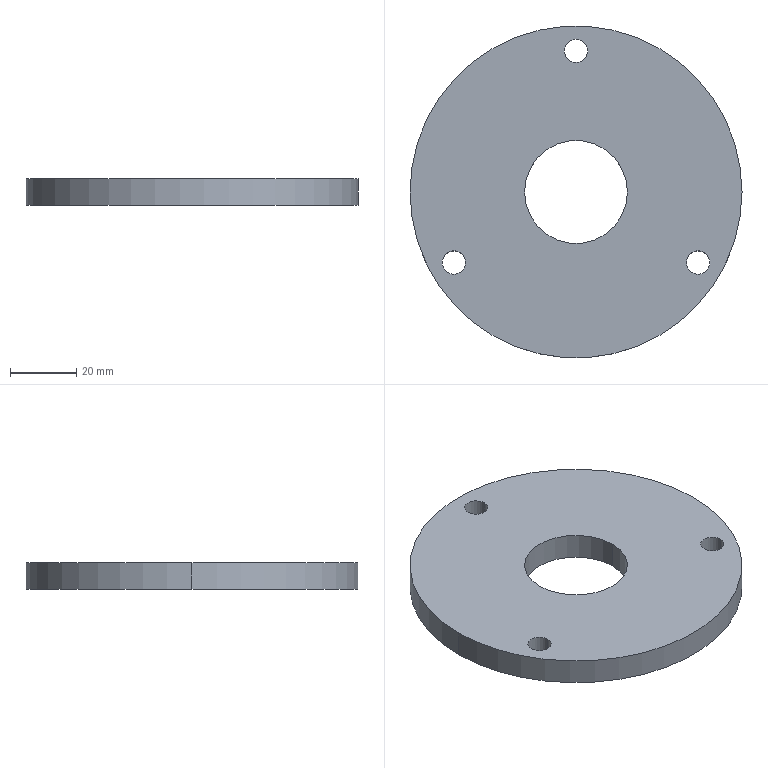Part | SolidWorks | features Extrusion 1 | 1 solid | 12 faces | box 100 x 100 x 8 mm | volume 55870 mm3 | cylinder 10 | plane 2 | commonest cylinder face diameters 7 x6 31 x2 100 x2
STEP:
#1=CARTESIAN_POINT('',(-15.5,0.,8.));
#2=VERTEX_POINT('',#1);
#3=CARTESIAN_POINT('',(15.5,0.,8.));
#4=VERTEX_POINT('',#3);
#5=CARTESIAN_POINT('',(0.,0.,8.));
#6=DIRECTION('',(0.,0.,1.));
#7=DIRECTION('',(1.,0.,0.));
#8=AXIS2_PLACEMENT_3D('',#5,#6,#7);
#9=CIRCLE('',#8,15.5);
#10=EDGE_CURVE('',#2,#4,#9,.T.);
#11=ORIENTED_EDGE('',*,*,#10,.T.);
#12=CARTESIAN_POINT('',(15.5,0.,0.));
#13=VERTEX_POINT('',#12);
#14=CARTESIAN_POINT('',(15.5,0.,8.));
#15=DIRECTION('',(0.,0.,-1.));
#16=VECTOR('',#15,1000.);
#17=LINE('',#14,#16);
#18=EDGE_CURVE('',#4,#13,#17,.T.);
#19=ORIENTED_EDGE('',*,*,#18,.T.);
#20=CARTESIAN_POINT('',(-15.5,0.,0.));
#21=VERTEX_POINT('',#20);
#22=CARTESIAN_POINT('',(0.,0.,0.));
#23=DIRECTION('',(0.,0.,1.));
#24=DIRECTION('',(1.,0.,0.));
#25=AXIS2_PLACEMENT_3D('',#22,#23,#24);
#26=CIRCLE('',#25,15.5);
#27=EDGE_CURVE('',#21,#13,#26,.T.);
#28=ORIENTED_EDGE('',*,*,#27,.F.);
#29=CARTESIAN_POINT('',(-15.5,0.,8.));
#30=DIRECTION('',(0.,0.,-1.));
#31=VECTOR('',#30,1000.);
#32=LINE('',#29,#31);
#33=EDGE_CURVE('',#2,#21,#32,.T.);
#34=ORIENTED_EDGE('',*,*,#33,.F.);
#35=EDGE_LOOP('',(#11,#19,#28,#34));
#36=FACE_OUTER_BOUND('',#35,.T.);
#37=CARTESIAN_POINT('',(0.,0.,8.));
#38=DIRECTION('',(0.,0.,-1.));
#39=DIRECTION('',(-1.,0.,0.));
#40=AXIS2_PLACEMENT_3D('',#37,#38,#39);
#41=CYLINDRICAL_SURFACE('',#40,15.5);
#42=ADVANCED_FACE('',(#36),#41,.F.);
#43=CARTESIAN_POINT('',(33.306,-21.25,8.));
#44=VERTEX_POINT('',#43);
#45=CARTESIAN_POINT('',(40.306,-21.25,8.));
#46=VERTEX_POINT('',#45);
#47=CARTESIAN_POINT('',(36.806,-21.25,8.));
#48=DIRECTION('',(0.,0.,1.));
#49=DIRECTION('',(1.,0.,0.));
#50=AXIS2_PLACEMENT_3D('',#47,#48,#49);
#51=CIRCLE('',#50,3.5);
#52=EDGE_CURVE('',#44,#46,#51,.T.);
#53=ORIENTED_EDGE('',*,*,#52,.T.);
#54=CARTESIAN_POINT('',(40.306,-21.25,0.));
#55=VERTEX_POINT('',#54);
#56=CARTESIAN_POINT('',(40.306,-21.25,8.));
#57=DIRECTION('',(0.,0.,-1.));
#58=VECTOR('',#57,1000.);
#59=LINE('',#56,#58);
#60=EDGE_CURVE('',#46,#55,#59,.T.);
#61=ORIENTED_EDGE('',*,*,#60,.T.);
#62=CARTESIAN_POINT('',(33.306,-21.25,0.));
#63=VERTEX_POINT('',#62);
#64=CARTESIAN_POINT('',(36.806,-21.25,0.));
#65=DIRECTION('',(0.,0.,1.));
#66=DIRECTION('',(1.,0.,0.));
#67=AXIS2_PLACEMENT_3D('',#64,#65,#66);
#68=CIRCLE('',#67,3.5);
#69=EDGE_CURVE('',#63,#55,#68,.T.);
#70=ORIENTED_EDGE('',*,*,#69,.F.);
#71=CARTESIAN_POINT('',(33.306,-21.25,8.));
#72=DIRECTION('',(0.,0.,-1.));
#73=VECTOR('',#72,1000.);
#74=LINE('',#71,#73);
#75=EDGE_CURVE('',#44,#63,#74,.T.);
#76=ORIENTED_EDGE('',*,*,#75,.F.);
#77=EDGE_LOOP('',(#53,#61,#70,#76));
#78=FACE_OUTER_BOUND('',#77,.T.);
#79=CARTESIAN_POINT('',(36.806,-21.25,8.));
#80=DIRECTION('',(0.,0.,-1.));
#81=DIRECTION('',(-1.,0.,0.));
#82=AXIS2_PLACEMENT_3D('',#79,#80,#81);
#83=CYLINDRICAL_SURFACE('',#82,3.5);
#84=ADVANCED_FACE('',(#78),#83,.F.);
#85=CARTESIAN_POINT('',(-40.306,-21.25,8.));
#86=VERTEX_POINT('',#85);
#87=CARTESIAN_POINT('',(-33.306,-21.25,8.));
#88=VERTEX_POINT('',#87);
#89=CARTESIAN_POINT('',(-36.806,-21.25,8.));
#90=DIRECTION('',(0.,0.,1.));
#91=DIRECTION('',(1.,0.,0.));
#92=AXIS2_PLACEMENT_3D('',#89,#90,#91);
#93=CIRCLE('',#92,3.5);
#94=EDGE_CURVE('',#86,#88,#93,.T.);
#95=ORIENTED_EDGE('',*,*,#94,.T.);
#96=CARTESIAN_POINT('',(-33.306,-21.25,0.));
#97=VERTEX_POINT('',#96);
#98=CARTESIAN_POINT('',(-33.306,-21.25,8.));
#99=DIRECTION('',(0.,0.,-1.));
#100=VECTOR('',#99,1000.);
#101=LINE('',#98,#100);
#102=EDGE_CURVE('',#88,#97,#101,.T.);
#103=ORIENTED_EDGE('',*,*,#102,.T.);
#104=CARTESIAN_POINT('',(-40.306,-21.25,0.));
#105=VERTEX_POINT('',#104);
#106=CARTESIAN_POINT('',(-36.806,-21.25,0.));
#107=DIRECTION('',(0.,0.,1.));
#108=DIRECTION('',(1.,0.,0.));
#109=AXIS2_PLACEMENT_3D('',#106,#107,#108);
#110=CIRCLE('',#109,3.5);
#111=EDGE_CURVE('',#105,#97,#110,.T.);
#112=ORIENTED_EDGE('',*,*,#111,.F.);
#113=CARTESIAN_POINT('',(-40.306,-21.25,8.));
#114=DIRECTION('',(0.,0.,-1.));
#115=VECTOR('',#114,1000.);
#116=LINE('',#113,#115);
#117=EDGE_CURVE('',#86,#105,#116,.T.);
#118=ORIENTED_EDGE('',*,*,#117,.F.);
#119=EDGE_LOOP('',(#95,#103,#112,#118));
#120=FACE_OUTER_BOUND('',#119,.T.);
#121=CARTESIAN_POINT('',(-36.806,-21.25,8.));
#122=DIRECTION('',(0.,0.,-1.));
#123=DIRECTION('',(-1.,0.,0.));
#124=AXIS2_PLACEMENT_3D('',#121,#122,#123);
#125=CYLINDRICAL_SURFACE('',#124,3.5);
#126=ADVANCED_FACE('',(#120),#125,.F.);
#127=CARTESIAN_POINT('',(-3.5,42.5,8.));
#128=VERTEX_POINT('',#127);
#129=CARTESIAN_POINT('',(3.5,42.5,8.));
#130=VERTEX_POINT('',#129);
#131=CARTESIAN_POINT('',(0.,42.5,8.));
#132=DIRECTION('',(0.,0.,1.));
#133=DIRECTION('',(1.,0.,0.));
#134=AXIS2_PLACEMENT_3D('',#131,#132,#133);
#135=CIRCLE('',#134,3.5);
#136=EDGE_CURVE('',#128,#130,#135,.T.);
#137=ORIENTED_EDGE('',*,*,#136,.T.);
#138=CARTESIAN_POINT('',(3.5,42.5,0.));
#139=VERTEX_POINT('',#138);
#140=CARTESIAN_POINT('',(3.5,42.5,8.));
#141=DIRECTION('',(0.,0.,-1.));
#142=VECTOR('',#141,1000.);
#143=LINE('',#140,#142);
#144=EDGE_CURVE('',#130,#139,#143,.T.);
#145=ORIENTED_EDGE('',*,*,#144,.T.);
#146=CARTESIAN_POINT('',(-3.5,42.5,0.));
#147=VERTEX_POINT('',#146);
#148=CARTESIAN_POINT('',(0.,42.5,0.));
#149=DIRECTION('',(0.,0.,1.));
#150=DIRECTION('',(1.,0.,0.));
#151=AXIS2_PLACEMENT_3D('',#148,#149,#150);
#152=CIRCLE('',#151,3.5);
#153=EDGE_CURVE('',#147,#139,#152,.T.);
#154=ORIENTED_EDGE('',*,*,#153,.F.);
#155=CARTESIAN_POINT('',(-3.5,42.5,8.));
#156=DIRECTION('',(0.,0.,-1.));
#157=VECTOR('',#156,1000.);
#158=LINE('',#155,#157);
#159=EDGE_CURVE('',#128,#147,#158,.T.);
#160=ORIENTED_EDGE('',*,*,#159,.F.);
#161=EDGE_LOOP('',(#137,#145,#154,#160));
#162=FACE_OUTER_BOUND('',#161,.T.);
#163=CARTESIAN_POINT('',(0.,42.5,8.));
#164=DIRECTION('',(0.,0.,-1.));
#165=DIRECTION('',(-1.,0.,0.));
#166=AXIS2_PLACEMENT_3D('',#163,#164,#165);
#167=CYLINDRICAL_SURFACE('',#166,3.5);
#168=ADVANCED_FACE('',(#162),#167,.F.);
#169=CARTESIAN_POINT('',(50.,0.,8.));
#170=VERTEX_POINT('',#169);
#171=CARTESIAN_POINT('',(-50.,0.,8.));
#172=VERTEX_POINT('',#171);
#173=CARTESIAN_POINT('',(0.,0.,8.));
#174=DIRECTION('',(0.,0.,1.));
#175=DIRECTION('',(1.,0.,0.));
#176=AXIS2_PLACEMENT_3D('',#173,#174,#175);
#177=CIRCLE('',#176,50.);
#178=EDGE_CURVE('',#170,#172,#177,.T.);
#179=ORIENTED_EDGE('',*,*,#178,.F.);
#180=CARTESIAN_POINT('',(50.,0.,0.));
#181=VERTEX_POINT('',#180);
#182=CARTESIAN_POINT('',(50.,0.,8.));
#183=DIRECTION('',(0.,0.,-1.));
#184=VECTOR('',#183,1000.);
#185=LINE('',#182,#184);
#186=EDGE_CURVE('',#170,#181,#185,.T.);
#187=ORIENTED_EDGE('',*,*,#186,.T.);
#188=CARTESIAN_POINT('',(-50.,0.,0.));
#189=VERTEX_POINT('',#188);
#190=CARTESIAN_POINT('',(0.,0.,0.));
#191=DIRECTION('',(0.,0.,1.));
#192=DIRECTION('',(1.,0.,0.));
#193=AXIS2_PLACEMENT_3D('',#190,#191,#192);
#194=CIRCLE('',#193,50.);
#195=EDGE_CURVE('',#181,#189,#194,.T.);
#196=ORIENTED_EDGE('',*,*,#195,.T.);
#197=CARTESIAN_POINT('',(-50.,0.,8.));
#198=DIRECTION('',(0.,0.,-1.));
#199=VECTOR('',#198,1000.);
#200=LINE('',#197,#199);
#201=EDGE_CURVE('',#172,#189,#200,.T.);
#202=ORIENTED_EDGE('',*,*,#201,.F.);
#203=EDGE_LOOP('',(#179,#187,#196,#202));
#204=FACE_OUTER_BOUND('',#203,.T.);
#205=CARTESIAN_POINT('',(0.,0.,8.));
#206=DIRECTION('',(0.,0.,-1.));
#207=DIRECTION('',(-1.,0.,0.));
#208=AXIS2_PLACEMENT_3D('',#205,#206,#207);
#209=CYLINDRICAL_SURFACE('',#208,50.);
#210=ADVANCED_FACE('',(#204),#209,.T.);
#211=ORIENTED_EDGE('',*,*,#52,.F.);
#212=CARTESIAN_POINT('',(36.806,-21.25,8.));
#213=DIRECTION('',(0.,0.,1.));
#214=DIRECTION('',(1.,0.,0.));
#215=AXIS2_PLACEMENT_3D('',#212,#213,#214);
#216=CIRCLE('',#215,3.5);
#217=EDGE_CURVE('',#46,#44,#216,.T.);
#218=ORIENTED_EDGE('',*,*,#217,.F.);
#219=EDGE_LOOP('',(#211,#218));
#220=FACE_BOUND('',#219,.T.);
#221=ORIENTED_EDGE('',*,*,#136,.F.);
#222=CARTESIAN_POINT('',(0.,42.5,8.));
#223=DIRECTION('',(0.,0.,1.));
#224=DIRECTION('',(1.,0.,0.));
#225=AXIS2_PLACEMENT_3D('',#222,#223,#224);
#226=CIRCLE('',#225,3.5);
#227=EDGE_CURVE('',#130,#128,#226,.T.);
#228=ORIENTED_EDGE('',*,*,#227,.F.);
#229=EDGE_LOOP('',(#221,#228));
#230=FACE_BOUND('',#229,.T.);
#231=CARTESIAN_POINT('',(0.,0.,8.));
#232=DIRECTION('',(0.,0.,1.));
#233=DIRECTION('',(1.,0.,0.));
#234=AXIS2_PLACEMENT_3D('',#231,#232,#233);
#235=CIRCLE('',#234,50.);
#236=EDGE_CURVE('',#172,#170,#235,.T.);
#237=ORIENTED_EDGE('',*,*,#236,.T.);
#238=ORIENTED_EDGE('',*,*,#178,.T.);
#239=EDGE_LOOP('',(#237,#238));
#240=FACE_OUTER_BOUND('',#239,.T.);
#241=ORIENTED_EDGE('',*,*,#94,.F.);
#242=CARTESIAN_POINT('',(-36.806,-21.25,8.));
#243=DIRECTION('',(0.,0.,1.));
#244=DIRECTION('',(1.,0.,0.));
#245=AXIS2_PLACEMENT_3D('',#242,#243,#244);
#246=CIRCLE('',#245,3.5);
#247=EDGE_CURVE('',#88,#86,#246,.T.);
#248=ORIENTED_EDGE('',*,*,#247,.F.);
#249=EDGE_LOOP('',(#241,#248));
#250=FACE_BOUND('',#249,.T.);
#251=ORIENTED_EDGE('',*,*,#10,.F.);
#252=CARTESIAN_POINT('',(0.,0.,8.));
#253=DIRECTION('',(0.,0.,1.));
#254=DIRECTION('',(1.,0.,0.));
#255=AXIS2_PLACEMENT_3D('',#252,#253,#254);
#256=CIRCLE('',#255,15.5);
#257=EDGE_CURVE('',#4,#2,#256,.T.);
#258=ORIENTED_EDGE('',*,*,#257,.F.);
#259=EDGE_LOOP('',(#251,#258));
#260=FACE_BOUND('',#259,.T.);
#261=CARTESIAN_POINT('',(0.,0.,8.));
#262=DIRECTION('',(0.,0.,1.));
#263=DIRECTION('',(1.,0.,0.));
#264=AXIS2_PLACEMENT_3D('',#261,#262,#263);
#265=PLANE('',#264);
#266=ADVANCED_FACE('',(#220,#230,#240,#250,#260),#265,.T.);
#267=CARTESIAN_POINT('',(0.,0.,0.));
#268=DIRECTION('',(0.,0.,1.));
#269=DIRECTION('',(1.,0.,0.));
#270=AXIS2_PLACEMENT_3D('',#267,#268,#269);
#271=CIRCLE('',#270,50.);
#272=EDGE_CURVE('',#189,#181,#271,.T.);
#273=ORIENTED_EDGE('',*,*,#272,.F.);
#274=ORIENTED_EDGE('',*,*,#195,.F.);
#275=EDGE_LOOP('',(#273,#274));
#276=FACE_OUTER_BOUND('',#275,.T.);
#277=ORIENTED_EDGE('',*,*,#153,.T.);
#278=CARTESIAN_POINT('',(0.,42.5,0.));
#279=DIRECTION('',(0.,0.,1.));
#280=DIRECTION('',(1.,0.,0.));
#281=AXIS2_PLACEMENT_3D('',#278,#279,#280);
#282=CIRCLE('',#281,3.5);
#283=EDGE_CURVE('',#139,#147,#282,.T.);
#284=ORIENTED_EDGE('',*,*,#283,.T.);
#285=EDGE_LOOP('',(#277,#284));
#286=FACE_BOUND('',#285,.T.);
#287=ORIENTED_EDGE('',*,*,#111,.T.);
#288=CARTESIAN_POINT('',(-36.806,-21.25,0.));
#289=DIRECTION('',(0.,0.,1.));
#290=DIRECTION('',(1.,0.,0.));
#291=AXIS2_PLACEMENT_3D('',#288,#289,#290);
#292=CIRCLE('',#291,3.5);
#293=EDGE_CURVE('',#97,#105,#292,.T.);
#294=ORIENTED_EDGE('',*,*,#293,.T.);
#295=EDGE_LOOP('',(#287,#294));
#296=FACE_BOUND('',#295,.T.);
#297=ORIENTED_EDGE('',*,*,#69,.T.);
#298=CARTESIAN_POINT('',(36.806,-21.25,0.));
#299=DIRECTION('',(0.,0.,1.));
#300=DIRECTION('',(1.,0.,0.));
#301=AXIS2_PLACEMENT_3D('',#298,#299,#300);
#302=CIRCLE('',#301,3.5);
#303=EDGE_CURVE('',#55,#63,#302,.T.);
#304=ORIENTED_EDGE('',*,*,#303,.T.);
#305=EDGE_LOOP('',(#297,#304));
#306=FACE_BOUND('',#305,.T.);
#307=ORIENTED_EDGE('',*,*,#27,.T.);
#308=CARTESIAN_POINT('',(0.,0.,0.));
#309=DIRECTION('',(0.,0.,1.));
#310=DIRECTION('',(1.,0.,0.));
#311=AXIS2_PLACEMENT_3D('',#308,#309,#310);
#312=CIRCLE('',#311,15.5);
#313=EDGE_CURVE('',#13,#21,#312,.T.);
#314=ORIENTED_EDGE('',*,*,#313,.T.);
#315=EDGE_LOOP('',(#307,#314));
#316=FACE_BOUND('',#315,.T.);
#317=CARTESIAN_POINT('',(0.,0.,0.));
#318=DIRECTION('',(0.,0.,1.));
#319=DIRECTION('',(1.,0.,0.));
#320=AXIS2_PLACEMENT_3D('',#317,#318,#319);
#321=PLANE('',#320);
#322=ADVANCED_FACE('',(#276,#286,#296,#306,#316),#321,.F.);
#323=ORIENTED_EDGE('',*,*,#186,.F.);
#324=ORIENTED_EDGE('',*,*,#236,.F.);
#325=ORIENTED_EDGE('',*,*,#201,.T.);
#326=ORIENTED_EDGE('',*,*,#272,.T.);
#327=EDGE_LOOP('',(#323,#324,#325,#326));
#328=FACE_OUTER_BOUND('',#327,.T.);
#329=CARTESIAN_POINT('',(0.,0.,8.));
#330=DIRECTION('',(0.,0.,-1.));
#331=DIRECTION('',(-1.,0.,0.));
#332=AXIS2_PLACEMENT_3D('',#329,#330,#331);
#333=CYLINDRICAL_SURFACE('',#332,50.);
#334=ADVANCED_FACE('',(#328),#333,.T.);
#335=ORIENTED_EDGE('',*,*,#144,.F.);
#336=ORIENTED_EDGE('',*,*,#227,.T.);
#337=ORIENTED_EDGE('',*,*,#159,.T.);
#338=ORIENTED_EDGE('',*,*,#283,.F.);
#339=EDGE_LOOP('',(#335,#336,#337,#338));
#340=FACE_OUTER_BOUND('',#339,.T.);
#341=CARTESIAN_POINT('',(0.,42.5,8.));
#342=DIRECTION('',(0.,0.,-1.));
#343=DIRECTION('',(-1.,0.,0.));
#344=AXIS2_PLACEMENT_3D('',#341,#342,#343);
#345=CYLINDRICAL_SURFACE('',#344,3.5);
#346=ADVANCED_FACE('',(#340),#345,.F.);
#347=ORIENTED_EDGE('',*,*,#102,.F.);
#348=ORIENTED_EDGE('',*,*,#247,.T.);
#349=ORIENTED_EDGE('',*,*,#117,.T.);
#350=ORIENTED_EDGE('',*,*,#293,.F.);
#351=EDGE_LOOP('',(#347,#348,#349,#350));
#352=FACE_OUTER_BOUND('',#351,.T.);
#353=CARTESIAN_POINT('',(-36.806,-21.25,8.));
#354=DIRECTION('',(0.,0.,-1.));
#355=DIRECTION('',(-1.,0.,0.));
#356=AXIS2_PLACEMENT_3D('',#353,#354,#355);
#357=CYLINDRICAL_SURFACE('',#356,3.5);
#358=ADVANCED_FACE('',(#352),#357,.F.);
#359=ORIENTED_EDGE('',*,*,#60,.F.);
#360=ORIENTED_EDGE('',*,*,#217,.T.);
#361=ORIENTED_EDGE('',*,*,#75,.T.);
#362=ORIENTED_EDGE('',*,*,#303,.F.);
#363=EDGE_LOOP('',(#359,#360,#361,#362));
#364=FACE_OUTER_BOUND('',#363,.T.);
#365=CARTESIAN_POINT('',(36.806,-21.25,8.));
#366=DIRECTION('',(0.,0.,-1.));
#367=DIRECTION('',(-1.,0.,0.));
#368=AXIS2_PLACEMENT_3D('',#365,#366,#367);
#369=CYLINDRICAL_SURFACE('',#368,3.5);
#370=ADVANCED_FACE('',(#364),#369,.F.);
#371=ORIENTED_EDGE('',*,*,#18,.F.);
#372=ORIENTED_EDGE('',*,*,#257,.T.);
#373=ORIENTED_EDGE('',*,*,#33,.T.);
#374=ORIENTED_EDGE('',*,*,#313,.F.);
#375=EDGE_LOOP('',(#371,#372,#373,#374));
#376=FACE_OUTER_BOUND('',#375,.T.);
#377=CARTESIAN_POINT('',(0.,0.,8.));
#378=DIRECTION('',(0.,0.,-1.));
#379=DIRECTION('',(-1.,0.,0.));
#380=AXIS2_PLACEMENT_3D('',#377,#378,#379);
#381=CYLINDRICAL_SURFACE('',#380,15.5);
#382=ADVANCED_FACE('',(#376),#381,.F.);
#383=CLOSED_SHELL('',(#42,#84,#126,#168,#210,#266,#322,#334,#346,#358,#370,#382));
#384=MANIFOLD_SOLID_BREP('',#383);
#385=CARTESIAN_POINT('',(0.,0.,0.));
#386=DIRECTION('',(0.,0.,1.));
#387=DIRECTION('',(1.,0.,0.));
#388=AXIS2_PLACEMENT_3D('',#385,#386,#387);
#389=(LENGTH_UNIT()NAMED_UNIT(*)SI_UNIT(.MILLI.,.METRE.));
#390=UNCERTAINTY_MEASURE_WITH_UNIT(LENGTH_MEASURE(0.00001),#389,'','');
#391=(NAMED_UNIT(*)PLANE_ANGLE_UNIT()SI_UNIT($,.RADIAN.));
#392=(NAMED_UNIT(*)SI_UNIT($,.STERADIAN.)SOLID_ANGLE_UNIT());
#393=(GEOMETRIC_REPRESENTATION_CONTEXT(3)GLOBAL_UNCERTAINTY_ASSIGNED_CONTEXT((#390))GLOBAL_UNIT_ASSIGNED_CONTEXT((#389,#391,#392))REPRESENTATION_CONTEXT('',''));
#394=ADVANCED_BREP_SHAPE_REPRESENTATION('',(#384,#388),#393);